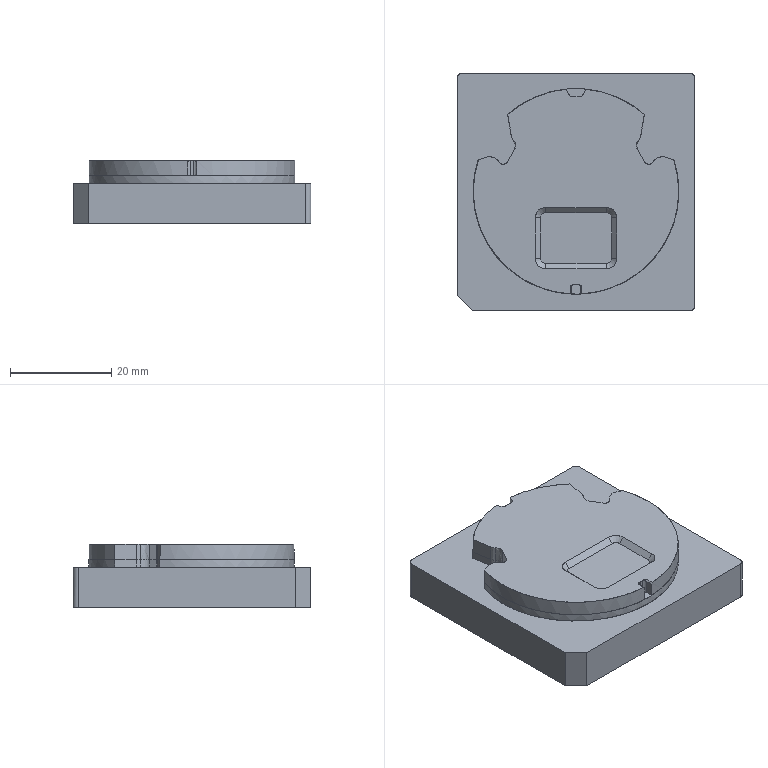CAM job | PowerMill | 3-axis milling, other | part box 47 x 47 x 12.511 mm
Tools:
number,name,type,diameter,tip_radius,length,cutting_length,overhang,flutes,holder,toolpaths_using
12,D2_3,end_mill,2.0,0.0,3.0,,2.0,1,D42L35,2
12,D2_1,end_mill,2.0,0.0,3.0,,2.0,1,D42L35,2
1,D10C,end_mill,10.0,0.0,60.0,,30.0,1,D42L35,2
15,D3C,end_mill,3.0,0.0,30.0,,15.0,1,D42L35,2
1,D10C_1_1,end_mill,10.0,0.0,60.0,,12.96,1,D42L35,6
15,D3C_1_1,end_mill,3.0,0.0,30.0,,4.56,1,D42L35,2
27,D1C_1_1,end_mill,1.0,0.0,4.72,,4.72,1,D42L35,1
3,D10_1_1,end_mill,10.0,0.0,60.0,,12.68,1,D42L35,8
14,D4_1_1,end_mill,4.0,0.0,30.0,,4.68,1,D42L35,1
12,D2_2_1,end_mill,2.0,0.0,4.68,,4.68,1,D42L35,1
8,D1_1_1,end_mill,1.0,0.0,4.68,,4.68,1,D42L35,1
13,Text_D4_1_1,taper_spherical,4.0,0.3,60.0,,4.76,1,D42L35,2
27,D1C_2_1,end_mill,1.0,0.0,4.56,,4.56,1,D42L35,1
14,D4_2_1,end_mill,4.0,0.0,30.0,,4.56,1,D42L35,1
12,D2_4_1,end_mill,2.0,0.0,4.56,,4.56,1,D42L35,1
8,D1_2_1,end_mill,1.0,0.0,3.28,,3.28,1,D42L35,1
Operations:
program,toolpath,strategy,tool,tool_number,tool_diameter,tip_radius,flutes,spindle_rpm,feed_cut,surface_speed_m_min_computed,feed_per_tooth_computed,tolerance,thickness,stepover,stepdown,cut_length,cut_time_min,total_time_min,workplane
02-B01-1-F,精公开粗01-扫面平行-D10C,raster_area_clear,D10C_1_1,1,10.0,0.0,1.0,8000.0,10000.0,251.33,1.25,0.03,0.28,6.0,1.0,578.16,0.058,0.065,
02-B01-1-F,精公开粗01-外形偏置-D10C,offset_area_clear,D10C_1_1,1,10.0,0.0,1.0,8000.0,10000.0,251.33,1.25,0.03,0.28,6.0,1.0,5136.259,0.514,0.5467,
02-B01-1-F,精公开粗01-基准台等高-D10C,constantz,D10C_1_1,1,10.0,0.0,1.0,8000.0,10000.0,251.33,1.25,0.03,0.07,5.0,0.4,4769.124,0.477,0.4869,
02-B01-1-F,精公再粗02-外形偏置-D3C,offset_area_clear,D3C_1_1,15,3.0,0.0,1.0,18000.0,5000.0,169.65,0.2778,0.03,0.0,2.0,1.0,5058.129,1.012,1.068,
02-B01-1-F,精公再粗03-外形偏置-D1C,offset_area_clear,D1C_1_1,27,1.0,0.0,1.0,22000.0,2000.0,69.12,0.0909,0.03,0.0,0.5,1.0,947.332,0.474,0.829,
02-B01-1-F,精公基准台01-平坦面平行-D10,raster_area_clear,D10_1_1,3,10.0,0.0,1.0,8500.0,600.0,267.04,0.0706,0.005,0.38,5.0,1.0,485.39,0.809,0.8407,
02-B01-1-F,精公基准台01-基准面偏置-D10,offset_area_clear,D10_1_1,3,10.0,0.0,1.0,8500.0,600.0,267.04,0.0706,0.005,0.38,5.0,1.0,270.886,0.452,0.4698,
02-B01-1-F,精公基准台01-外形侧光-D10,profile_area_clear,D10_1_1,3,10.0,0.0,1.0,8500.0,600.0,267.04,0.0706,0.005,-0.07,0.08,1.0,324.892,0.541,0.5618,
02-B01-1-F,精公基准台01-基准台侧光-D10,profile_area_clear,D10_1_1,3,10.0,0.0,1.0,8500.0,600.0,267.04,0.0706,0.005,0.0,0.08,1.0,433.233,0.722,0.7865,
02-B01-1-F,精公精光01-等高-D4,constantz,D4_1_1,14,4.0,0.0,1.0,18000.0,2000.0,226.19,0.1111,0.005,-0.075,5.0,0.04,17754.563,8.877,9.113,
02-B01-1-F,精公精光02-等高-D2,constantz,D2_1,12,2.0,0.0,1.0,18000.0,1500.0,113.1,0.0833,0.005,-0.075,5.0,0.01,4430.553,2.954,3.069,
02-B01-1-F,精公精光02-平坦面偏置-D2,offset_area_clear,D2_1,12,2.0,0.0,1.0,18000.0,600.0,113.1,0.0333,0.005,-0.07,1.0,1.0,114.735,0.191,0.214,
02-B01-1-F,精公精光03-等高-D2,constantz,D2_2_1,12,2.0,0.0,1.0,18000.0,1500.0,113.1,0.0833,0.005,-0.075,5.0,0.01,2677.39,1.785,2.518,
02-B01-1-F,精公精光04-等高-D1,constantz,D1_1_1,8,1.0,0.0,1.0,20000.0,1000.0,62.83,0.05,0.005,-0.075,5.0,0.01,2396.484,2.397,2.924,
02-B01-1-F,精公刻字01-刻字-Text_D4,pattern,Text_D4_1_1,13,4.0,0.3,1.0,15000.0,1000.0,188.5,0.0667,0.005,0.0,5.0,1.0,24.452,0.025,0.0407,
02-B01-1-R,粗公开粗01-扫面平行-D10C,raster_area_clear,D10C_1_1,1,10.0,0.0,1.0,8000.0,10000.0,251.33,1.25,0.03,0.15,6.0,1.0,575.3,0.058,0.0648,
02-B01-1-R,粗公开粗01-外形偏置-D10C,offset_area_clear,D10C_1_1,1,10.0,0.0,1.0,8000.0,10000.0,251.33,1.25,0.03,0.15,6.0,1.0,4688.698,0.469,0.4996,
02-B01-1-R,粗公开粗01-基准台等高-D10C,constantz,D10C_1_1,1,10.0,0.0,1.0,8000.0,10000.0,251.33,1.25,0.03,0.07,5.0,0.4,4769.124,0.477,0.4869,
02-B01-1-R,粗公再粗02-外形偏置-D3C,offset_area_clear,D3C_1_1,15,3.0,0.0,1.0,18000.0,5000.0,169.65,0.2778,0.03,-0.13,2.0,1.0,5063.748,1.013,1.073,
02-B01-1-R,粗公再粗03-外形偏置-D1C,offset_area_clear,D1C_2_1,27,1.0,0.0,1.0,22000.0,2000.0,69.12,0.0909,0.03,-0.13,0.5,1.0,1086.084,0.543,0.9364,
02-B01-1-R,粗公基准台01-平坦面平行-D10,raster_area_clear,D10_1_1,3,10.0,0.0,1.0,8500.0,600.0,267.04,0.0706,0.01,0.25,5.0,1.0,475.037,0.792,0.8093,
02-B01-1-R,粗公基准台01-基准面偏置-D10,offset_area_clear,D10_1_1,3,10.0,0.0,1.0,8500.0,600.0,267.04,0.0706,0.01,0.25,5.0,1.0,269.192,0.449,0.467,
02-B01-1-R,粗公基准台01-外形侧光-D10,profile_area_clear,D10_1_1,3,10.0,0.0,1.0,8500.0,600.0,267.04,0.0706,0.01,-0.2,0.08,1.0,323.49,0.539,0.5594,
02-B01-1-R,粗公基准台01-基准台侧光-D10,profile_area_clear,D10_1_1,3,10.0,0.0,1.0,8500.0,600.0,267.04,0.0706,0.01,0.0,0.08,1.0,433.218,0.722,0.7865,
02-B01-1-R,粗公精光01-等高-D4,constantz,D4_2_1,14,4.0,0.0,1.0,18000.0,2000.0,226.19,0.1111,0.01,-0.205,5.0,0.048,14251.374,7.126,7.316,
02-B01-1-R,粗公精光02-等高-D2,constantz,D2_3,12,2.0,0.0,1.0,18000.0,1500.0,113.1,0.0833,0.01,-0.205,5.0,0.01,4512.685,3.009,3.124,
02-B01-1-R,粗公精光02-平坦面偏置-D2,offset_area_clear,D2_3,12,2.0,0.0,1.0,18000.0,600.0,113.1,0.0333,0.01,-0.2,1.0,1.0,118.845,0.198,0.2209,
02-B01-1-R,粗公精光03-等高-D2,constantz,D2_4_1,12,2.0,0.0,1.0,18000.0,1500.0,113.1,0.0833,0.01,-0.205,5.0,0.01,3572.827,2.382,3.154,
02-B01-1-R,粗公精光04-等高-D1,constantz,D1_2_1,8,1.0,0.0,1.0,20000.0,1000.0,62.83,0.05,0.01,-0.205,5.0,0.01,1153.638,1.154,1.393,
02-B01-1-R,粗公刻字01-刻字-Text_D4,pattern,Text_D4_1_1,13,4.0,0.3,1.0,15000.0,1000.0,188.5,0.0667,0.01,0.0,5.0,1.0,24.162,0.024,0.0396,
,精公开粗01-外形偏置-D10C_Reference,offset_area_clear,D10C,1,10.0,0.0,1.0,8000.0,10000.0,251.33,1.25,0.03,0.28,6.0,1.0,12838.293,1.284,1.361,
,精公再粗02-外形偏置-D3C_Reference,offset_area_clear,D3C,15,3.0,0.0,1.0,18000.0,5000.0,169.65,0.2778,0.03,0.0,2.0,1.0,15819.185,3.164,3.326,
,粗公开粗01-外形偏置-D10C_Reference,offset_area_clear,D10C,1,10.0,0.0,1.0,8000.0,10000.0,251.33,1.25,0.03,0.15,6.0,1.0,12359.264,1.236,1.31,
,粗公再粗02-外形偏置-D3C_Reference,offset_area_clear,D3C,15,3.0,0.0,1.0,18000.0,5000.0,169.65,0.2778,0.03,-0.13,2.0,1.0,14812.927,2.963,3.122,